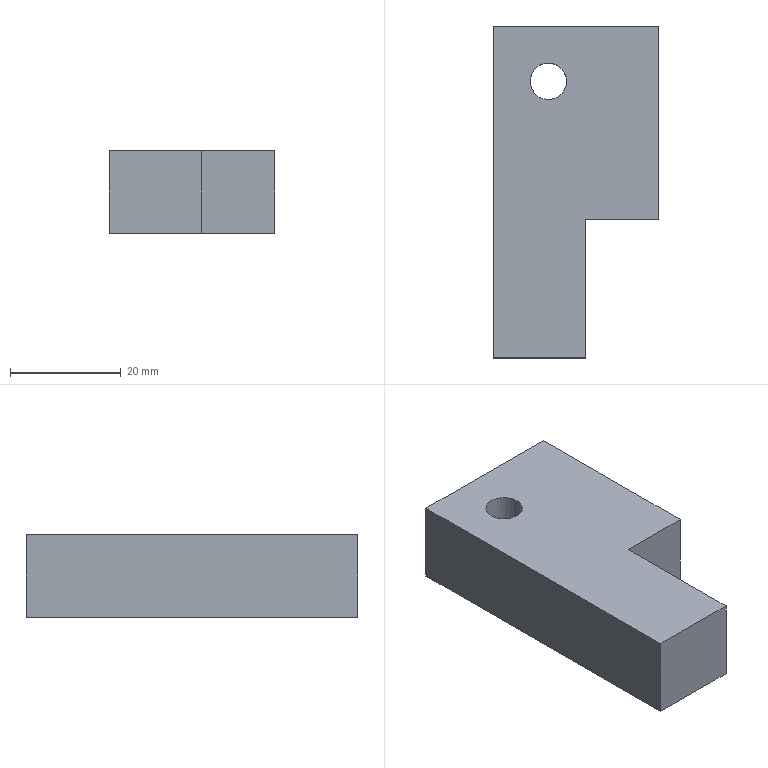Part | NX | features 5003_211_Plate 2 | 1 solid | 13 faces | box 30 x 60 x 15 mm | volume 20902 mm3 | plane 8 | cylinder 3 | cone 2 | commonest cylinder face diameters 5 x2 6.6 x1
STEP:
#1=CARTESIAN_POINT('',(-196.775,-597.1,-69.5));
#2=VERTEX_POINT('',#1);
#3=CARTESIAN_POINT('',(-210.045,-597.1,-69.5));
#4=VERTEX_POINT('',#3);
#5=CARTESIAN_POINT('',(-210.045,-597.1,-69.5));
#6=DIRECTION('',(-1.,0.,0.));
#7=VECTOR('',#6,1000.);
#8=LINE('',#5,#7);
#9=EDGE_CURVE('',#2,#4,#8,.T.);
#10=ORIENTED_EDGE('',*,*,#9,.T.);
#11=CARTESIAN_POINT('',(-210.045,-597.1,-84.5));
#12=VERTEX_POINT('',#11);
#13=CARTESIAN_POINT('',(-210.045,-597.1,-84.5));
#14=DIRECTION('',(0.,0.,1.));
#15=VECTOR('',#14,1000.);
#16=LINE('',#13,#15);
#17=EDGE_CURVE('',#12,#4,#16,.T.);
#18=ORIENTED_EDGE('',*,*,#17,.F.);
#19=CARTESIAN_POINT('',(-196.775,-597.1,-84.5));
#20=VERTEX_POINT('',#19);
#21=CARTESIAN_POINT('',(-210.045,-597.1,-84.5));
#22=DIRECTION('',(-1.,0.,0.));
#23=VECTOR('',#22,1000.);
#24=LINE('',#21,#23);
#25=EDGE_CURVE('',#20,#12,#24,.T.);
#26=ORIENTED_EDGE('',*,*,#25,.F.);
#27=CARTESIAN_POINT('',(-196.775,-597.1,-84.5));
#28=DIRECTION('',(0.,0.,1.));
#29=VECTOR('',#28,1000.);
#30=LINE('',#27,#29);
#31=EDGE_CURVE('',#20,#2,#30,.T.);
#32=ORIENTED_EDGE('',*,*,#31,.T.);
#33=EDGE_LOOP('',(#10,#18,#26,#32));
#34=FACE_BOUND('',#33,.T.);
#35=CARTESIAN_POINT('',(-210.045,-597.1,-84.5));
#36=DIRECTION('',(0.,1.,0.));
#37=DIRECTION('',(1.,0.,0.));
#38=AXIS2_PLACEMENT_3D('',#35,#36,#37);
#39=PLANE('',#38);
#40=ADVANCED_FACE('',(#34),#39,.F.);
#41=CARTESIAN_POINT('',(-210.045,-622.1,-69.5));
#42=VERTEX_POINT('',#41);
#43=CARTESIAN_POINT('',(-210.045,-622.1,-69.5));
#44=DIRECTION('',(0.,-1.,0.));
#45=VECTOR('',#44,1000.);
#46=LINE('',#43,#45);
#47=EDGE_CURVE('',#4,#42,#46,.T.);
#48=ORIENTED_EDGE('',*,*,#47,.T.);
#49=CARTESIAN_POINT('',(-210.045,-622.1,-84.5));
#50=VERTEX_POINT('',#49);
#51=CARTESIAN_POINT('',(-210.045,-622.1,-84.5));
#52=DIRECTION('',(0.,0.,1.));
#53=VECTOR('',#52,1000.);
#54=LINE('',#51,#53);
#55=EDGE_CURVE('',#50,#42,#54,.T.);
#56=ORIENTED_EDGE('',*,*,#55,.F.);
#57=CARTESIAN_POINT('',(-210.045,-622.1,-84.5));
#58=DIRECTION('',(0.,-1.,0.));
#59=VECTOR('',#58,1000.);
#60=LINE('',#57,#59);
#61=EDGE_CURVE('',#12,#50,#60,.T.);
#62=ORIENTED_EDGE('',*,*,#61,.F.);
#63=ORIENTED_EDGE('',*,*,#17,.T.);
#64=EDGE_LOOP('',(#48,#56,#62,#63));
#65=FACE_BOUND('',#64,.T.);
#66=CARTESIAN_POINT('',(-210.045,-622.1,-84.5));
#67=DIRECTION('',(-1.,0.,0.));
#68=DIRECTION('',(0.,1.,0.));
#69=AXIS2_PLACEMENT_3D('',#66,#67,#68);
#70=PLANE('',#69);
#71=ADVANCED_FACE('',(#65),#70,.F.);
#72=CARTESIAN_POINT('',(-226.775,-622.1,-69.5));
#73=VERTEX_POINT('',#72);
#74=CARTESIAN_POINT('',(-226.775,-622.1,-69.5));
#75=DIRECTION('',(-1.,0.,0.));
#76=VECTOR('',#75,1000.);
#77=LINE('',#74,#76);
#78=EDGE_CURVE('',#42,#73,#77,.T.);
#79=ORIENTED_EDGE('',*,*,#78,.T.);
#80=CARTESIAN_POINT('',(-226.775,-622.1,-84.5));
#81=VERTEX_POINT('',#80);
#82=CARTESIAN_POINT('',(-226.775,-622.1,-84.5));
#83=DIRECTION('',(0.,0.,1.));
#84=VECTOR('',#83,1000.);
#85=LINE('',#82,#84);
#86=EDGE_CURVE('',#81,#73,#85,.T.);
#87=ORIENTED_EDGE('',*,*,#86,.F.);
#88=CARTESIAN_POINT('',(-226.775,-622.1,-84.5));
#89=DIRECTION('',(-1.,0.,0.));
#90=VECTOR('',#89,1000.);
#91=LINE('',#88,#90);
#92=EDGE_CURVE('',#50,#81,#91,.T.);
#93=ORIENTED_EDGE('',*,*,#92,.F.);
#94=ORIENTED_EDGE('',*,*,#55,.T.);
#95=EDGE_LOOP('',(#79,#87,#93,#94));
#96=FACE_BOUND('',#95,.T.);
#97=CARTESIAN_POINT('',(-226.775,-622.1,-84.5));
#98=DIRECTION('',(0.,1.,0.));
#99=DIRECTION('',(1.,0.,0.));
#100=AXIS2_PLACEMENT_3D('',#97,#98,#99);
#101=PLANE('',#100);
#102=ADVANCED_FACE('',(#96),#101,.F.);
#103=CARTESIAN_POINT('',(-226.775,-562.1,-69.5));
#104=VERTEX_POINT('',#103);
#105=CARTESIAN_POINT('',(-226.775,-562.1,-69.5));
#106=DIRECTION('',(0.,1.,0.));
#107=VECTOR('',#106,1000.);
#108=LINE('',#105,#107);
#109=EDGE_CURVE('',#73,#104,#108,.T.);
#110=ORIENTED_EDGE('',*,*,#109,.T.);
#111=CARTESIAN_POINT('',(-226.775,-562.1,-84.5));
#112=VERTEX_POINT('',#111);
#113=CARTESIAN_POINT('',(-226.775,-562.1,-84.5));
#114=DIRECTION('',(0.,0.,1.));
#115=VECTOR('',#114,1000.);
#116=LINE('',#113,#115);
#117=EDGE_CURVE('',#112,#104,#116,.T.);
#118=ORIENTED_EDGE('',*,*,#117,.F.);
#119=CARTESIAN_POINT('',(-226.775,-562.1,-84.5));
#120=DIRECTION('',(0.,1.,0.));
#121=VECTOR('',#120,1000.);
#122=LINE('',#119,#121);
#123=EDGE_CURVE('',#81,#112,#122,.T.);
#124=ORIENTED_EDGE('',*,*,#123,.F.);
#125=ORIENTED_EDGE('',*,*,#86,.T.);
#126=EDGE_LOOP('',(#110,#118,#124,#125));
#127=FACE_BOUND('',#126,.T.);
#128=CARTESIAN_POINT('',(-226.775,-562.1,-84.5));
#129=DIRECTION('',(1.,0.,0.));
#130=DIRECTION('',(0.,-1.,0.));
#131=AXIS2_PLACEMENT_3D('',#128,#129,#130);
#132=PLANE('',#131);
#133=ADVANCED_FACE('',(#127),#132,.F.);
#134=CARTESIAN_POINT('',(-196.775,-562.1,-69.5));
#135=VERTEX_POINT('',#134);
#136=CARTESIAN_POINT('',(-196.775,-562.1,-69.5));
#137=DIRECTION('',(1.,0.,0.));
#138=VECTOR('',#137,1000.);
#139=LINE('',#136,#138);
#140=EDGE_CURVE('',#104,#135,#139,.T.);
#141=ORIENTED_EDGE('',*,*,#140,.T.);
#142=CARTESIAN_POINT('',(-196.775,-562.1,-84.5));
#143=VERTEX_POINT('',#142);
#144=CARTESIAN_POINT('',(-196.775,-562.1,-84.5));
#145=DIRECTION('',(0.,0.,1.));
#146=VECTOR('',#145,1000.);
#147=LINE('',#144,#146);
#148=EDGE_CURVE('',#143,#135,#147,.T.);
#149=ORIENTED_EDGE('',*,*,#148,.F.);
#150=CARTESIAN_POINT('',(-196.775,-562.1,-84.5));
#151=DIRECTION('',(1.,0.,0.));
#152=VECTOR('',#151,1000.);
#153=LINE('',#150,#152);
#154=EDGE_CURVE('',#112,#143,#153,.T.);
#155=ORIENTED_EDGE('',*,*,#154,.F.);
#156=ORIENTED_EDGE('',*,*,#117,.T.);
#157=EDGE_LOOP('',(#141,#149,#155,#156));
#158=FACE_BOUND('',#157,.T.);
#159=CARTESIAN_POINT('',(-196.775,-562.1,-84.5));
#160=DIRECTION('',(0.,-1.,0.));
#161=DIRECTION('',(-1.,0.,0.));
#162=AXIS2_PLACEMENT_3D('',#159,#160,#161);
#163=PLANE('',#162);
#164=ADVANCED_FACE('',(#158),#163,.F.);
#165=CARTESIAN_POINT('',(-196.775,-572.1,-77.));
#166=VERTEX_POINT('',#165);
#167=CARTESIAN_POINT('',(-196.775,-569.6,-77.));
#168=DIRECTION('',(1.,0.,0.));
#169=DIRECTION('',(0.,-1.,0.));
#170=AXIS2_PLACEMENT_3D('',#167,#168,#169);
#171=CIRCLE('',#170,2.5);
#172=EDGE_CURVE('',#166,#166,#171,.T.);
#173=ORIENTED_EDGE('',*,*,#172,.F.);
#174=EDGE_LOOP('',(#173));
#175=FACE_BOUND('',#174,.T.);
#176=CARTESIAN_POINT('',(-196.775,-592.1,-77.));
#177=VERTEX_POINT('',#176);
#178=CARTESIAN_POINT('',(-196.775,-589.6,-77.));
#179=DIRECTION('',(1.,0.,0.));
#180=DIRECTION('',(0.,-1.,0.));
#181=AXIS2_PLACEMENT_3D('',#178,#179,#180);
#182=CIRCLE('',#181,2.5);
#183=EDGE_CURVE('',#177,#177,#182,.T.);
#184=ORIENTED_EDGE('',*,*,#183,.F.);
#185=EDGE_LOOP('',(#184));
#186=FACE_BOUND('',#185,.T.);
#187=CARTESIAN_POINT('',(-196.775,-597.1,-69.5));
#188=DIRECTION('',(0.,-1.,0.));
#189=VECTOR('',#188,1000.);
#190=LINE('',#187,#189);
#191=EDGE_CURVE('',#135,#2,#190,.T.);
#192=ORIENTED_EDGE('',*,*,#191,.T.);
#193=ORIENTED_EDGE('',*,*,#31,.F.);
#194=CARTESIAN_POINT('',(-196.775,-597.1,-84.5));
#195=DIRECTION('',(0.,-1.,0.));
#196=VECTOR('',#195,1000.);
#197=LINE('',#194,#196);
#198=EDGE_CURVE('',#143,#20,#197,.T.);
#199=ORIENTED_EDGE('',*,*,#198,.F.);
#200=ORIENTED_EDGE('',*,*,#148,.T.);
#201=EDGE_LOOP('',(#192,#193,#199,#200));
#202=FACE_BOUND('',#201,.T.);
#203=CARTESIAN_POINT('',(-196.775,-597.1,-84.5));
#204=DIRECTION('',(-1.,0.,0.));
#205=DIRECTION('',(0.,1.,0.));
#206=AXIS2_PLACEMENT_3D('',#203,#204,#205);
#207=PLANE('',#206);
#208=ADVANCED_FACE('',(#175,#186,#202),#207,.F.);
#209=CARTESIAN_POINT('',(-213.475,-572.1,-84.5));
#210=VERTEX_POINT('',#209);
#211=CARTESIAN_POINT('',(-216.775,-572.1,-84.5));
#212=DIRECTION('',(0.,0.,1.));
#213=DIRECTION('',(1.,0.,0.));
#214=AXIS2_PLACEMENT_3D('',#211,#212,#213);
#215=CIRCLE('',#214,3.3);
#216=EDGE_CURVE('',#210,#210,#215,.T.);
#217=ORIENTED_EDGE('',*,*,#216,.T.);
#218=EDGE_LOOP('',(#217));
#219=FACE_BOUND('',#218,.T.);
#220=ORIENTED_EDGE('',*,*,#25,.T.);
#221=ORIENTED_EDGE('',*,*,#61,.T.);
#222=ORIENTED_EDGE('',*,*,#92,.T.);
#223=ORIENTED_EDGE('',*,*,#123,.T.);
#224=ORIENTED_EDGE('',*,*,#154,.T.);
#225=ORIENTED_EDGE('',*,*,#198,.T.);
#226=EDGE_LOOP('',(#220,#221,#222,#223,#224,#225));
#227=FACE_BOUND('',#226,.T.);
#228=CARTESIAN_POINT('',(-196.775,-597.1,-84.5));
#229=DIRECTION('',(0.,0.,1.));
#230=DIRECTION('',(1.,0.,0.));
#231=AXIS2_PLACEMENT_3D('',#228,#229,#230);
#232=PLANE('',#231);
#233=ADVANCED_FACE('',(#219,#227),#232,.F.);
#234=CARTESIAN_POINT('',(-213.475,-572.1,-69.5));
#235=VERTEX_POINT('',#234);
#236=CARTESIAN_POINT('',(-216.775,-572.1,-69.5));
#237=DIRECTION('',(0.,0.,1.));
#238=DIRECTION('',(1.,0.,0.));
#239=AXIS2_PLACEMENT_3D('',#236,#237,#238);
#240=CIRCLE('',#239,3.3);
#241=EDGE_CURVE('',#235,#235,#240,.T.);
#242=ORIENTED_EDGE('',*,*,#241,.F.);
#243=EDGE_LOOP('',(#242));
#244=FACE_BOUND('',#243,.T.);
#245=ORIENTED_EDGE('',*,*,#9,.F.);
#246=ORIENTED_EDGE('',*,*,#191,.F.);
#247=ORIENTED_EDGE('',*,*,#140,.F.);
#248=ORIENTED_EDGE('',*,*,#109,.F.);
#249=ORIENTED_EDGE('',*,*,#78,.F.);
#250=ORIENTED_EDGE('',*,*,#47,.F.);
#251=EDGE_LOOP('',(#245,#246,#247,#248,#249,#250));
#252=FACE_BOUND('',#251,.T.);
#253=CARTESIAN_POINT('',(-196.775,-597.1,-69.5));
#254=DIRECTION('',(0.,0.,1.));
#255=DIRECTION('',(1.,0.,0.));
#256=AXIS2_PLACEMENT_3D('',#253,#254,#255);
#257=PLANE('',#256);
#258=ADVANCED_FACE('',(#244,#252),#257,.T.);
#259=CARTESIAN_POINT('',(-213.277,-589.6,-77.));
#260=VERTEX_POINT('',#259);
#261=VERTEX_LOOP('',#260);
#262=FACE_BOUND('',#261,.T.);
#263=CARTESIAN_POINT('',(-211.775,-592.1,-77.));
#264=VERTEX_POINT('',#263);
#265=CARTESIAN_POINT('',(-211.775,-589.6,-77.));
#266=DIRECTION('',(1.,0.,0.));
#267=DIRECTION('',(0.,-1.,0.));
#268=AXIS2_PLACEMENT_3D('',#265,#266,#267);
#269=CIRCLE('',#268,2.5);
#270=EDGE_CURVE('',#264,#264,#269,.T.);
#271=ORIENTED_EDGE('',*,*,#270,.T.);
#272=EDGE_LOOP('',(#271));
#273=FACE_BOUND('',#272,.T.);
#274=CARTESIAN_POINT('',(-211.775,-589.6,-77.));
#275=DIRECTION('',(1.,0.,0.));
#276=DIRECTION('',(0.,-1.,0.));
#277=AXIS2_PLACEMENT_3D('',#274,#275,#276);
#278=CONICAL_SURFACE('',#277,2.5,1.03);
#279=ADVANCED_FACE('',(#262,#273),#278,.F.);
#280=ORIENTED_EDGE('',*,*,#270,.F.);
#281=EDGE_LOOP('',(#280));
#282=FACE_BOUND('',#281,.T.);
#283=ORIENTED_EDGE('',*,*,#183,.T.);
#284=EDGE_LOOP('',(#283));
#285=FACE_BOUND('',#284,.T.);
#286=CARTESIAN_POINT('',(-196.775,-589.6,-77.));
#287=DIRECTION('',(1.,0.,0.));
#288=DIRECTION('',(0.,-1.,0.));
#289=AXIS2_PLACEMENT_3D('',#286,#287,#288);
#290=CYLINDRICAL_SURFACE('',#289,2.5);
#291=ADVANCED_FACE('',(#282,#285),#290,.F.);
#292=CARTESIAN_POINT('',(-213.277,-569.6,-77.));
#293=VERTEX_POINT('',#292);
#294=VERTEX_LOOP('',#293);
#295=FACE_BOUND('',#294,.T.);
#296=CARTESIAN_POINT('',(-211.775,-572.1,-77.));
#297=VERTEX_POINT('',#296);
#298=CARTESIAN_POINT('',(-211.775,-569.6,-77.));
#299=DIRECTION('',(1.,0.,0.));
#300=DIRECTION('',(0.,-1.,0.));
#301=AXIS2_PLACEMENT_3D('',#298,#299,#300);
#302=CIRCLE('',#301,2.5);
#303=EDGE_CURVE('',#297,#297,#302,.T.);
#304=ORIENTED_EDGE('',*,*,#303,.T.);
#305=EDGE_LOOP('',(#304));
#306=FACE_BOUND('',#305,.T.);
#307=CARTESIAN_POINT('',(-211.775,-569.6,-77.));
#308=DIRECTION('',(1.,0.,0.));
#309=DIRECTION('',(0.,-1.,0.));
#310=AXIS2_PLACEMENT_3D('',#307,#308,#309);
#311=CONICAL_SURFACE('',#310,2.5,1.03);
#312=ADVANCED_FACE('',(#295,#306),#311,.F.);
#313=ORIENTED_EDGE('',*,*,#303,.F.);
#314=EDGE_LOOP('',(#313));
#315=FACE_BOUND('',#314,.T.);
#316=ORIENTED_EDGE('',*,*,#172,.T.);
#317=EDGE_LOOP('',(#316));
#318=FACE_BOUND('',#317,.T.);
#319=CARTESIAN_POINT('',(-196.775,-569.6,-77.));
#320=DIRECTION('',(1.,0.,0.));
#321=DIRECTION('',(0.,-1.,0.));
#322=AXIS2_PLACEMENT_3D('',#319,#320,#321);
#323=CYLINDRICAL_SURFACE('',#322,2.5);
#324=ADVANCED_FACE('',(#315,#318),#323,.F.);
#325=ORIENTED_EDGE('',*,*,#216,.F.);
#326=EDGE_LOOP('',(#325));
#327=FACE_BOUND('',#326,.T.);
#328=ORIENTED_EDGE('',*,*,#241,.T.);
#329=EDGE_LOOP('',(#328));
#330=FACE_BOUND('',#329,.T.);
#331=CARTESIAN_POINT('',(-216.775,-572.1,-69.5));
#332=DIRECTION('',(0.,0.,1.));
#333=DIRECTION('',(1.,0.,0.));
#334=AXIS2_PLACEMENT_3D('',#331,#332,#333);
#335=CYLINDRICAL_SURFACE('',#334,3.3);
#336=ADVANCED_FACE('',(#327,#330),#335,.F.);
#337=CLOSED_SHELL('',(#40,#71,#102,#133,#164,#208,#233,#258,#279,#291,#312,#324,#336));
#338=MANIFOLD_SOLID_BREP('',#337);
#339=(LENGTH_UNIT()NAMED_UNIT(*)SI_UNIT(.MILLI.,.METRE.));
#340=UNCERTAINTY_MEASURE_WITH_UNIT(LENGTH_MEASURE(0.00001),#339,'','');
#341=(NAMED_UNIT(*)PLANE_ANGLE_UNIT()SI_UNIT($,.RADIAN.));
#342=(NAMED_UNIT(*)SI_UNIT($,.STERADIAN.)SOLID_ANGLE_UNIT());
#343=(GEOMETRIC_REPRESENTATION_CONTEXT(3)GLOBAL_UNCERTAINTY_ASSIGNED_CONTEXT((#340))GLOBAL_UNIT_ASSIGNED_CONTEXT((#339,#341,#342))REPRESENTATION_CONTEXT('',''));
#344=ADVANCED_BREP_SHAPE_REPRESENTATION('',(#338),#343);